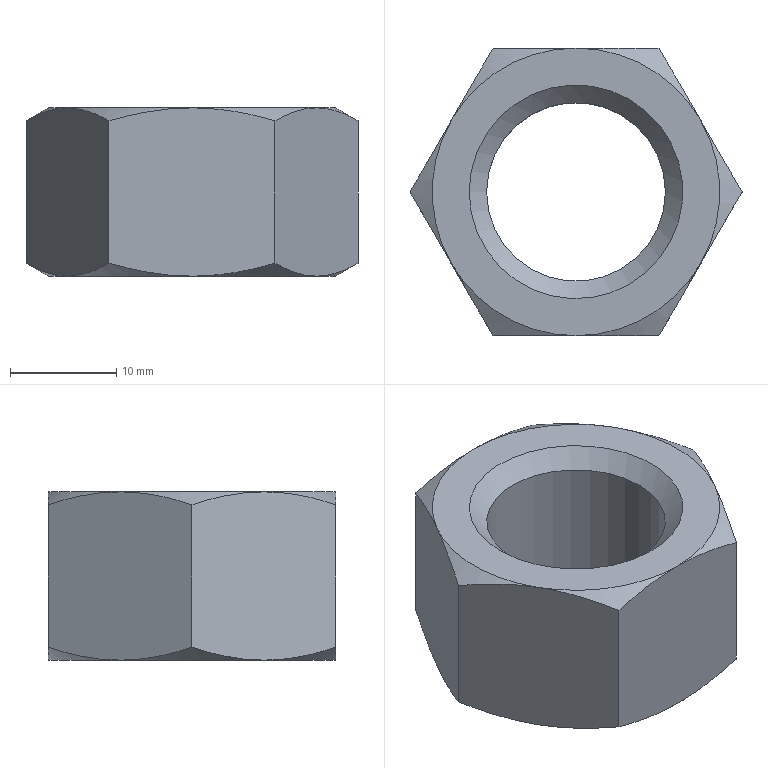Part | NX | features META 3, SKETCH 3, DATUM_CSYS 2, EXTRUDE 2, SWP104 2, CHAMFER 1, LINE 1, SYMBOLIC_THREAD 1, THREADS 1 | 1 solid | 23 faces | box 31.177 x 27 x 15.8 mm | volume 6286 mm3 | cone 14 | plane 8 | cylinder 1 | commonest cylinder face diameters 16.782 x1
STEP:
#1=CARTESIAN_POINT('',(-7.794,13.5,14.594));
#2=VERTEX_POINT('',#1);
#3=CARTESIAN_POINT('',(-7.794,13.5,1.206));
#4=VERTEX_POINT('',#3);
#5=CARTESIAN_POINT('',(-7.794,13.5,15.8));
#6=DIRECTION('',(0.,0.,-1.));
#7=VECTOR('',#6,1000.);
#8=LINE('',#5,#7);
#9=EDGE_CURVE('',#2,#4,#8,.T.);
#10=ORIENTED_EDGE('',*,*,#9,.T.);
#11=CARTESIAN_POINT('',(-11.691,6.75,0.));
#12=VERTEX_POINT('',#11);
#13=CARTESIAN_POINT('',(-7.794,13.5,1.206));
#14=CARTESIAN_POINT('',(-9.069,11.292,0.4696));
#15=CARTESIAN_POINT('',(-10.363,9.05,0.));
#16=CARTESIAN_POINT('',(-11.691,6.75,0.));
#17=B_SPLINE_CURVE_WITH_KNOTS('',3,(#13,#14,#15,#16),.UNSPECIFIED.,.F.,.F.,(4,4),(0.000000238,0.007887),.UNSPECIFIED.);
#18=EDGE_CURVE('',#4,#12,#17,.T.);
#19=ORIENTED_EDGE('',*,*,#18,.T.);
#20=CARTESIAN_POINT('',(-15.588,0.,1.206));
#21=VERTEX_POINT('',#20);
#22=CARTESIAN_POINT('',(-11.691,6.75,0.));
#23=CARTESIAN_POINT('',(-13.014,4.459,0.));
#24=CARTESIAN_POINT('',(-14.317,2.203,0.4715));
#25=CARTESIAN_POINT('',(-15.588,0.,1.206));
#26=B_SPLINE_CURVE_WITH_KNOTS('',3,(#22,#23,#24,#25),.UNSPECIFIED.,.F.,.F.,(4,4),(0.007887,0.01574),.UNSPECIFIED.);
#27=EDGE_CURVE('',#12,#21,#26,.T.);
#28=ORIENTED_EDGE('',*,*,#27,.T.);
#29=CARTESIAN_POINT('',(-15.588,0.,14.594));
#30=VERTEX_POINT('',#29);
#31=CARTESIAN_POINT('',(-15.588,0.,15.8));
#32=DIRECTION('',(0.,0.,-1.));
#33=VECTOR('',#32,1000.);
#34=LINE('',#31,#33);
#35=EDGE_CURVE('',#30,#21,#34,.T.);
#36=ORIENTED_EDGE('',*,*,#35,.F.);
#37=CARTESIAN_POINT('',(-11.691,6.75,15.8));
#38=VERTEX_POINT('',#37);
#39=CARTESIAN_POINT('',(-11.691,6.75,15.8));
#40=CARTESIAN_POINT('',(-13.014,4.459,15.8));
#41=CARTESIAN_POINT('',(-14.317,2.203,15.329));
#42=CARTESIAN_POINT('',(-15.588,0.,14.594));
#43=B_SPLINE_CURVE_WITH_KNOTS('',3,(#39,#40,#41,#42),.UNSPECIFIED.,.F.,.F.,(4,4),(0.007887,0.01574),.UNSPECIFIED.);
#44=EDGE_CURVE('',#38,#30,#43,.T.);
#45=ORIENTED_EDGE('',*,*,#44,.F.);
#46=CARTESIAN_POINT('',(-7.794,13.5,14.594));
#47=CARTESIAN_POINT('',(-9.069,11.292,15.33));
#48=CARTESIAN_POINT('',(-10.363,9.05,15.8));
#49=CARTESIAN_POINT('',(-11.691,6.75,15.8));
#50=B_SPLINE_CURVE_WITH_KNOTS('',3,(#46,#47,#48,#49),.UNSPECIFIED.,.F.,.F.,(4,4),(0.000000238,0.007887),.UNSPECIFIED.);
#51=EDGE_CURVE('',#2,#38,#50,.T.);
#52=ORIENTED_EDGE('',*,*,#51,.F.);
#53=EDGE_LOOP('',(#10,#19,#28,#36,#45,#52));
#54=FACE_BOUND('',#53,.T.);
#55=CARTESIAN_POINT('',(-15.588,0.,15.8));
#56=DIRECTION('',(-0.866,0.5,0.));
#57=DIRECTION('',(-0.5,-0.866,0.));
#58=AXIS2_PLACEMENT_3D('',#55,#56,#57);
#59=PLANE('',#58);
#60=ADVANCED_FACE('',(#54),#59,.T.);
#61=CARTESIAN_POINT('',(7.794,13.5,14.594));
#62=VERTEX_POINT('',#61);
#63=CARTESIAN_POINT('',(7.794,13.5,1.206));
#64=VERTEX_POINT('',#63);
#65=CARTESIAN_POINT('',(7.794,13.5,15.8));
#66=DIRECTION('',(0.,0.,-1.));
#67=VECTOR('',#66,1000.);
#68=LINE('',#65,#67);
#69=EDGE_CURVE('',#62,#64,#68,.T.);
#70=ORIENTED_EDGE('',*,*,#69,.T.);
#71=CARTESIAN_POINT('',(0.,13.5,0.));
#72=VERTEX_POINT('',#71);
#73=CARTESIAN_POINT('',(0.,13.5,0.));
#74=CARTESIAN_POINT('',(2.636,13.5,0.));
#75=CARTESIAN_POINT('',(5.274,13.5,0.4781));
#76=CARTESIAN_POINT('',(7.794,13.5,1.206));
#77=B_SPLINE_CURVE_WITH_KNOTS('',3,(#73,#74,#75,#76),.UNSPECIFIED.,.F.,.F.,(4,4),(0.02179,0.02968),.UNSPECIFIED.);
#78=EDGE_CURVE('',#64,#72,#77,.F.);
#79=ORIENTED_EDGE('',*,*,#78,.T.);
#80=CARTESIAN_POINT('',(-7.794,13.5,1.206));
#81=CARTESIAN_POINT('',(-5.259,13.5,0.4739));
#82=CARTESIAN_POINT('',(-2.634,13.5,0.));
#83=CARTESIAN_POINT('',(0.,13.5,0.));
#84=B_SPLINE_CURVE_WITH_KNOTS('',3,(#80,#81,#82,#83),.UNSPECIFIED.,.F.,.F.,(4,4),(0.01391,0.02179),.UNSPECIFIED.);
#85=EDGE_CURVE('',#72,#4,#84,.F.);
#86=ORIENTED_EDGE('',*,*,#85,.T.);
#87=ORIENTED_EDGE('',*,*,#9,.F.);
#88=CARTESIAN_POINT('',(0.,13.5,15.8));
#89=VERTEX_POINT('',#88);
#90=CARTESIAN_POINT('',(-7.794,13.5,14.594));
#91=CARTESIAN_POINT('',(-5.259,13.5,15.326));
#92=CARTESIAN_POINT('',(-2.634,13.5,15.8));
#93=CARTESIAN_POINT('',(0.,13.5,15.8));
#94=B_SPLINE_CURVE_WITH_KNOTS('',3,(#90,#91,#92,#93),.UNSPECIFIED.,.F.,.F.,(4,4),(0.01391,0.02179),.UNSPECIFIED.);
#95=EDGE_CURVE('',#89,#2,#94,.F.);
#96=ORIENTED_EDGE('',*,*,#95,.F.);
#97=CARTESIAN_POINT('',(0.,13.5,15.8));
#98=CARTESIAN_POINT('',(2.636,13.5,15.8));
#99=CARTESIAN_POINT('',(5.274,13.5,15.322));
#100=CARTESIAN_POINT('',(7.794,13.5,14.594));
#101=B_SPLINE_CURVE_WITH_KNOTS('',3,(#97,#98,#99,#100),.UNSPECIFIED.,.F.,.F.,(4,4),(0.02179,0.02968),.UNSPECIFIED.);
#102=EDGE_CURVE('',#62,#89,#101,.F.);
#103=ORIENTED_EDGE('',*,*,#102,.F.);
#104=EDGE_LOOP('',(#70,#79,#86,#87,#96,#103));
#105=FACE_BOUND('',#104,.T.);
#106=CARTESIAN_POINT('',(-7.794,13.5,15.8));
#107=DIRECTION('',(0.,1.,0.));
#108=DIRECTION('',(0.,0.,1.));
#109=AXIS2_PLACEMENT_3D('',#106,#107,#108);
#110=PLANE('',#109);
#111=ADVANCED_FACE('',(#105),#110,.T.);
#112=CARTESIAN_POINT('',(15.588,0.,14.594));
#113=VERTEX_POINT('',#112);
#114=CARTESIAN_POINT('',(15.588,0.,1.206));
#115=VERTEX_POINT('',#114);
#116=CARTESIAN_POINT('',(15.588,0.,15.8));
#117=DIRECTION('',(0.,0.,-1.));
#118=VECTOR('',#117,1000.);
#119=LINE('',#116,#118);
#120=EDGE_CURVE('',#113,#115,#119,.T.);
#121=ORIENTED_EDGE('',*,*,#120,.T.);
#122=CARTESIAN_POINT('',(11.691,6.75,0.));
#123=VERTEX_POINT('',#122);
#124=CARTESIAN_POINT('',(15.588,0.,1.206));
#125=CARTESIAN_POINT('',(14.313,2.208,0.4696));
#126=CARTESIAN_POINT('',(13.019,4.45,0.));
#127=CARTESIAN_POINT('',(11.691,6.75,0.));
#128=B_SPLINE_CURVE_WITH_KNOTS('',3,(#124,#125,#126,#127),.UNSPECIFIED.,.F.,.F.,(4,4),(0.000000238,0.007887),.UNSPECIFIED.);
#129=EDGE_CURVE('',#115,#123,#128,.T.);
#130=ORIENTED_EDGE('',*,*,#129,.T.);
#131=CARTESIAN_POINT('',(11.691,6.75,0.));
#132=CARTESIAN_POINT('',(10.368,9.041,0.));
#133=CARTESIAN_POINT('',(9.066,11.297,0.4715));
#134=CARTESIAN_POINT('',(7.794,13.5,1.206));
#135=B_SPLINE_CURVE_WITH_KNOTS('',3,(#131,#132,#133,#134),.UNSPECIFIED.,.F.,.F.,(4,4),(0.007887,0.01574),.UNSPECIFIED.);
#136=EDGE_CURVE('',#123,#64,#135,.T.);
#137=ORIENTED_EDGE('',*,*,#136,.T.);
#138=ORIENTED_EDGE('',*,*,#69,.F.);
#139=CARTESIAN_POINT('',(11.691,6.75,15.8));
#140=VERTEX_POINT('',#139);
#141=CARTESIAN_POINT('',(11.691,6.75,15.8));
#142=CARTESIAN_POINT('',(10.368,9.041,15.8));
#143=CARTESIAN_POINT('',(9.066,11.297,15.329));
#144=CARTESIAN_POINT('',(7.794,13.5,14.594));
#145=B_SPLINE_CURVE_WITH_KNOTS('',3,(#141,#142,#143,#144),.UNSPECIFIED.,.F.,.F.,(4,4),(0.007887,0.01574),.UNSPECIFIED.);
#146=EDGE_CURVE('',#140,#62,#145,.T.);
#147=ORIENTED_EDGE('',*,*,#146,.F.);
#148=CARTESIAN_POINT('',(15.588,0.,14.594));
#149=CARTESIAN_POINT('',(14.313,2.208,15.33));
#150=CARTESIAN_POINT('',(13.019,4.45,15.8));
#151=CARTESIAN_POINT('',(11.691,6.75,15.8));
#152=B_SPLINE_CURVE_WITH_KNOTS('',3,(#148,#149,#150,#151),.UNSPECIFIED.,.F.,.F.,(4,4),(0.000000238,0.007887),.UNSPECIFIED.);
#153=EDGE_CURVE('',#113,#140,#152,.T.);
#154=ORIENTED_EDGE('',*,*,#153,.F.);
#155=EDGE_LOOP('',(#121,#130,#137,#138,#147,#154));
#156=FACE_BOUND('',#155,.T.);
#157=CARTESIAN_POINT('',(7.794,13.5,15.8));
#158=DIRECTION('',(0.866,0.5,0.));
#159=DIRECTION('',(-0.5,0.866,0.));
#160=AXIS2_PLACEMENT_3D('',#157,#158,#159);
#161=PLANE('',#160);
#162=ADVANCED_FACE('',(#156),#161,.T.);
#163=CARTESIAN_POINT('',(7.794,-13.5,14.594));
#164=VERTEX_POINT('',#163);
#165=CARTESIAN_POINT('',(7.794,-13.5,1.206));
#166=VERTEX_POINT('',#165);
#167=CARTESIAN_POINT('',(7.794,-13.5,15.8));
#168=DIRECTION('',(0.,0.,-1.));
#169=VECTOR('',#168,1000.);
#170=LINE('',#167,#169);
#171=EDGE_CURVE('',#164,#166,#170,.T.);
#172=ORIENTED_EDGE('',*,*,#171,.T.);
#173=CARTESIAN_POINT('',(11.691,-6.75,0.));
#174=VERTEX_POINT('',#173);
#175=CARTESIAN_POINT('',(7.794,-13.5,1.206));
#176=CARTESIAN_POINT('',(9.069,-11.292,0.4696));
#177=CARTESIAN_POINT('',(10.363,-9.05,0.));
#178=CARTESIAN_POINT('',(11.691,-6.75,0.));
#179=B_SPLINE_CURVE_WITH_KNOTS('',3,(#175,#176,#177,#178),.UNSPECIFIED.,.F.,.F.,(4,4),(0.000000238,0.007887),.UNSPECIFIED.);
#180=EDGE_CURVE('',#166,#174,#179,.T.);
#181=ORIENTED_EDGE('',*,*,#180,.T.);
#182=CARTESIAN_POINT('',(11.691,-6.75,0.));
#183=CARTESIAN_POINT('',(13.014,-4.459,0.));
#184=CARTESIAN_POINT('',(14.317,-2.203,0.4715));
#185=CARTESIAN_POINT('',(15.588,0.,1.206));
#186=B_SPLINE_CURVE_WITH_KNOTS('',3,(#182,#183,#184,#185),.UNSPECIFIED.,.F.,.F.,(4,4),(0.007887,0.01574),.UNSPECIFIED.);
#187=EDGE_CURVE('',#174,#115,#186,.T.);
#188=ORIENTED_EDGE('',*,*,#187,.T.);
#189=ORIENTED_EDGE('',*,*,#120,.F.);
#190=CARTESIAN_POINT('',(11.691,-6.75,15.8));
#191=VERTEX_POINT('',#190);
#192=CARTESIAN_POINT('',(11.691,-6.75,15.8));
#193=CARTESIAN_POINT('',(13.014,-4.459,15.8));
#194=CARTESIAN_POINT('',(14.317,-2.203,15.329));
#195=CARTESIAN_POINT('',(15.588,0.,14.594));
#196=B_SPLINE_CURVE_WITH_KNOTS('',3,(#192,#193,#194,#195),.UNSPECIFIED.,.F.,.F.,(4,4),(0.007887,0.01574),.UNSPECIFIED.);
#197=EDGE_CURVE('',#191,#113,#196,.T.);
#198=ORIENTED_EDGE('',*,*,#197,.F.);
#199=CARTESIAN_POINT('',(7.794,-13.5,14.594));
#200=CARTESIAN_POINT('',(9.069,-11.292,15.33));
#201=CARTESIAN_POINT('',(10.363,-9.05,15.8));
#202=CARTESIAN_POINT('',(11.691,-6.75,15.8));
#203=B_SPLINE_CURVE_WITH_KNOTS('',3,(#199,#200,#201,#202),.UNSPECIFIED.,.F.,.F.,(4,4),(0.000000238,0.007887),.UNSPECIFIED.);
#204=EDGE_CURVE('',#164,#191,#203,.T.);
#205=ORIENTED_EDGE('',*,*,#204,.F.);
#206=EDGE_LOOP('',(#172,#181,#188,#189,#198,#205));
#207=FACE_BOUND('',#206,.T.);
#208=CARTESIAN_POINT('',(15.588,0.,15.8));
#209=DIRECTION('',(0.866,-0.5,0.));
#210=DIRECTION('',(0.5,0.866,0.));
#211=AXIS2_PLACEMENT_3D('',#208,#209,#210);
#212=PLANE('',#211);
#213=ADVANCED_FACE('',(#207),#212,.T.);
#214=CARTESIAN_POINT('',(-7.794,-13.5,14.594));
#215=VERTEX_POINT('',#214);
#216=CARTESIAN_POINT('',(-7.794,-13.5,1.206));
#217=VERTEX_POINT('',#216);
#218=CARTESIAN_POINT('',(-7.794,-13.5,15.8));
#219=DIRECTION('',(0.,0.,-1.));
#220=VECTOR('',#219,1000.);
#221=LINE('',#218,#220);
#222=EDGE_CURVE('',#215,#217,#221,.T.);
#223=ORIENTED_EDGE('',*,*,#222,.T.);
#224=CARTESIAN_POINT('',(0.,-13.5,0.));
#225=VERTEX_POINT('',#224);
#226=CARTESIAN_POINT('',(-7.794,-13.5,1.206));
#227=CARTESIAN_POINT('',(-5.259,-13.5,0.4739));
#228=CARTESIAN_POINT('',(-2.634,-13.5,0.));
#229=CARTESIAN_POINT('',(0.,-13.5,0.));
#230=B_SPLINE_CURVE_WITH_KNOTS('',3,(#226,#227,#228,#229),.UNSPECIFIED.,.F.,.F.,(4,4),(0.01391,0.02179),.UNSPECIFIED.);
#231=EDGE_CURVE('',#217,#225,#230,.T.);
#232=ORIENTED_EDGE('',*,*,#231,.T.);
#233=CARTESIAN_POINT('',(0.,-13.5,0.));
#234=CARTESIAN_POINT('',(2.636,-13.5,0.));
#235=CARTESIAN_POINT('',(5.274,-13.5,0.4781));
#236=CARTESIAN_POINT('',(7.794,-13.5,1.206));
#237=B_SPLINE_CURVE_WITH_KNOTS('',3,(#233,#234,#235,#236),.UNSPECIFIED.,.F.,.F.,(4,4),(0.02179,0.02968),.UNSPECIFIED.);
#238=EDGE_CURVE('',#225,#166,#237,.T.);
#239=ORIENTED_EDGE('',*,*,#238,.T.);
#240=ORIENTED_EDGE('',*,*,#171,.F.);
#241=CARTESIAN_POINT('',(0.,-13.5,15.8));
#242=VERTEX_POINT('',#241);
#243=CARTESIAN_POINT('',(0.,-13.5,15.8));
#244=CARTESIAN_POINT('',(2.636,-13.5,15.8));
#245=CARTESIAN_POINT('',(5.274,-13.5,15.322));
#246=CARTESIAN_POINT('',(7.794,-13.5,14.594));
#247=B_SPLINE_CURVE_WITH_KNOTS('',3,(#243,#244,#245,#246),.UNSPECIFIED.,.F.,.F.,(4,4),(0.02179,0.02968),.UNSPECIFIED.);
#248=EDGE_CURVE('',#242,#164,#247,.T.);
#249=ORIENTED_EDGE('',*,*,#248,.F.);
#250=CARTESIAN_POINT('',(-7.794,-13.5,14.594));
#251=CARTESIAN_POINT('',(-5.259,-13.5,15.326));
#252=CARTESIAN_POINT('',(-2.634,-13.5,15.8));
#253=CARTESIAN_POINT('',(0.,-13.5,15.8));
#254=B_SPLINE_CURVE_WITH_KNOTS('',3,(#250,#251,#252,#253),.UNSPECIFIED.,.F.,.F.,(4,4),(0.01391,0.02179),.UNSPECIFIED.);
#255=EDGE_CURVE('',#215,#242,#254,.T.);
#256=ORIENTED_EDGE('',*,*,#255,.F.);
#257=EDGE_LOOP('',(#223,#232,#239,#240,#249,#256));
#258=FACE_BOUND('',#257,.T.);
#259=CARTESIAN_POINT('',(7.794,-13.5,15.8));
#260=DIRECTION('',(0.,-1.,0.));
#261=DIRECTION('',(0.,0.,-1.));
#262=AXIS2_PLACEMENT_3D('',#259,#260,#261);
#263=PLANE('',#262);
#264=ADVANCED_FACE('',(#258),#263,.T.);
#265=ORIENTED_EDGE('',*,*,#35,.T.);
#266=CARTESIAN_POINT('',(-11.691,-6.75,0.));
#267=VERTEX_POINT('',#266);
#268=CARTESIAN_POINT('',(-15.588,0.,1.206));
#269=CARTESIAN_POINT('',(-14.313,-2.208,0.4696));
#270=CARTESIAN_POINT('',(-13.019,-4.45,0.));
#271=CARTESIAN_POINT('',(-11.691,-6.75,0.));
#272=B_SPLINE_CURVE_WITH_KNOTS('',3,(#268,#269,#270,#271),.UNSPECIFIED.,.F.,.F.,(4,4),(0.000000238,0.007887),.UNSPECIFIED.);
#273=EDGE_CURVE('',#21,#267,#272,.T.);
#274=ORIENTED_EDGE('',*,*,#273,.T.);
#275=CARTESIAN_POINT('',(-11.691,-6.75,0.));
#276=CARTESIAN_POINT('',(-10.368,-9.041,0.));
#277=CARTESIAN_POINT('',(-9.066,-11.297,0.4715));
#278=CARTESIAN_POINT('',(-7.794,-13.5,1.206));
#279=B_SPLINE_CURVE_WITH_KNOTS('',3,(#275,#276,#277,#278),.UNSPECIFIED.,.F.,.F.,(4,4),(0.007887,0.01574),.UNSPECIFIED.);
#280=EDGE_CURVE('',#267,#217,#279,.T.);
#281=ORIENTED_EDGE('',*,*,#280,.T.);
#282=ORIENTED_EDGE('',*,*,#222,.F.);
#283=CARTESIAN_POINT('',(-11.691,-6.75,15.8));
#284=VERTEX_POINT('',#283);
#285=CARTESIAN_POINT('',(-11.691,-6.75,15.8));
#286=CARTESIAN_POINT('',(-10.368,-9.041,15.8));
#287=CARTESIAN_POINT('',(-9.066,-11.297,15.329));
#288=CARTESIAN_POINT('',(-7.794,-13.5,14.594));
#289=B_SPLINE_CURVE_WITH_KNOTS('',3,(#285,#286,#287,#288),.UNSPECIFIED.,.F.,.F.,(4,4),(0.007887,0.01574),.UNSPECIFIED.);
#290=EDGE_CURVE('',#284,#215,#289,.T.);
#291=ORIENTED_EDGE('',*,*,#290,.F.);
#292=CARTESIAN_POINT('',(-15.588,0.,14.594));
#293=CARTESIAN_POINT('',(-14.313,-2.208,15.33));
#294=CARTESIAN_POINT('',(-13.019,-4.45,15.8));
#295=CARTESIAN_POINT('',(-11.691,-6.75,15.8));
#296=B_SPLINE_CURVE_WITH_KNOTS('',3,(#292,#293,#294,#295),.UNSPECIFIED.,.F.,.F.,(4,4),(0.000000238,0.007887),.UNSPECIFIED.);
#297=EDGE_CURVE('',#30,#284,#296,.T.);
#298=ORIENTED_EDGE('',*,*,#297,.F.);
#299=EDGE_LOOP('',(#265,#274,#281,#282,#291,#298));
#300=FACE_BOUND('',#299,.T.);
#301=CARTESIAN_POINT('',(-7.794,-13.5,15.8));
#302=DIRECTION('',(-0.866,-0.5,0.));
#303=DIRECTION('',(0.5,-0.866,0.));
#304=AXIS2_PLACEMENT_3D('',#301,#302,#303);
#305=PLANE('',#304);
#306=ADVANCED_FACE('',(#300),#305,.T.);
#307=CARTESIAN_POINT('',(-10.027,0.,0.));
#308=VERTEX_POINT('',#307);
#309=CARTESIAN_POINT('',(0.,0.,0.));
#310=DIRECTION('',(0.,0.,-1.));
#311=DIRECTION('',(-1.,0.,0.));
#312=AXIS2_PLACEMENT_3D('',#309,#310,#311);
#313=CIRCLE('',#312,10.027);
#314=EDGE_CURVE('',#308,#308,#313,.F.);
#315=ORIENTED_EDGE('',*,*,#314,.T.);
#316=EDGE_LOOP('',(#315));
#317=FACE_BOUND('',#316,.T.);
#318=CARTESIAN_POINT('',(0.,0.,0.));
#319=DIRECTION('',(0.,0.,-1.));
#320=DIRECTION('',(-1.,0.,0.));
#321=AXIS2_PLACEMENT_3D('',#318,#319,#320);
#322=CIRCLE('',#321,13.5);
#323=EDGE_CURVE('',#267,#12,#322,.T.);
#324=ORIENTED_EDGE('',*,*,#323,.T.);
#325=CARTESIAN_POINT('',(0.,0.,0.));
#326=DIRECTION('',(0.,0.,-1.));
#327=DIRECTION('',(-1.,0.,0.));
#328=AXIS2_PLACEMENT_3D('',#325,#326,#327);
#329=CIRCLE('',#328,13.5);
#330=EDGE_CURVE('',#12,#72,#329,.T.);
#331=ORIENTED_EDGE('',*,*,#330,.T.);
#332=CARTESIAN_POINT('',(0.,0.,0.));
#333=DIRECTION('',(0.,0.,-1.));
#334=DIRECTION('',(-1.,0.,0.));
#335=AXIS2_PLACEMENT_3D('',#332,#333,#334);
#336=CIRCLE('',#335,13.5);
#337=EDGE_CURVE('',#72,#123,#336,.T.);
#338=ORIENTED_EDGE('',*,*,#337,.T.);
#339=CARTESIAN_POINT('',(0.,0.,0.));
#340=DIRECTION('',(0.,0.,-1.));
#341=DIRECTION('',(-1.,0.,0.));
#342=AXIS2_PLACEMENT_3D('',#339,#340,#341);
#343=CIRCLE('',#342,13.5);
#344=EDGE_CURVE('',#123,#174,#343,.T.);
#345=ORIENTED_EDGE('',*,*,#344,.T.);
#346=CARTESIAN_POINT('',(0.,0.,0.));
#347=DIRECTION('',(0.,0.,-1.));
#348=DIRECTION('',(-1.,0.,0.));
#349=AXIS2_PLACEMENT_3D('',#346,#347,#348);
#350=CIRCLE('',#349,13.5);
#351=EDGE_CURVE('',#174,#225,#350,.T.);
#352=ORIENTED_EDGE('',*,*,#351,.T.);
#353=CARTESIAN_POINT('',(0.,0.,0.));
#354=DIRECTION('',(0.,0.,-1.));
#355=DIRECTION('',(-1.,0.,0.));
#356=AXIS2_PLACEMENT_3D('',#353,#354,#355);
#357=CIRCLE('',#356,13.5);
#358=EDGE_CURVE('',#225,#267,#357,.T.);
#359=ORIENTED_EDGE('',*,*,#358,.T.);
#360=EDGE_LOOP('',(#324,#331,#338,#345,#352,#359));
#361=FACE_BOUND('',#360,.T.);
#362=CARTESIAN_POINT('',(-7.794,13.5,0.));
#363=DIRECTION('',(0.,0.,-1.));
#364=DIRECTION('',(-1.,0.,0.));
#365=AXIS2_PLACEMENT_3D('',#362,#363,#364);
#366=PLANE('',#365);
#367=ADVANCED_FACE('',(#317,#361),#366,.T.);
#368=CARTESIAN_POINT('',(-10.027,0.,15.8));
#369=VERTEX_POINT('',#368);
#370=CARTESIAN_POINT('',(0.,0.,15.8));
#371=DIRECTION('',(0.,0.,-1.));
#372=DIRECTION('',(-1.,0.,0.));
#373=AXIS2_PLACEMENT_3D('',#370,#371,#372);
#374=CIRCLE('',#373,10.027);
#375=EDGE_CURVE('',#369,#369,#374,.T.);
#376=ORIENTED_EDGE('',*,*,#375,.T.);
#377=EDGE_LOOP('',(#376));
#378=FACE_BOUND('',#377,.T.);
#379=CARTESIAN_POINT('',(0.,0.,15.8));
#380=DIRECTION('',(0.,0.,-1.));
#381=DIRECTION('',(-1.,0.,0.));
#382=AXIS2_PLACEMENT_3D('',#379,#380,#381);
#383=CIRCLE('',#382,13.5);
#384=EDGE_CURVE('',#38,#89,#383,.T.);
#385=ORIENTED_EDGE('',*,*,#384,.F.);
#386=CARTESIAN_POINT('',(0.,0.,15.8));
#387=DIRECTION('',(0.,0.,-1.));
#388=DIRECTION('',(-1.,0.,0.));
#389=AXIS2_PLACEMENT_3D('',#386,#387,#388);
#390=CIRCLE('',#389,13.5);
#391=EDGE_CURVE('',#284,#38,#390,.T.);
#392=ORIENTED_EDGE('',*,*,#391,.F.);
#393=CARTESIAN_POINT('',(0.,0.,15.8));
#394=DIRECTION('',(0.,0.,-1.));
#395=DIRECTION('',(-1.,0.,0.));
#396=AXIS2_PLACEMENT_3D('',#393,#394,#395);
#397=CIRCLE('',#396,13.5);
#398=EDGE_CURVE('',#242,#284,#397,.T.);
#399=ORIENTED_EDGE('',*,*,#398,.F.);
#400=CARTESIAN_POINT('',(0.,0.,15.8));
#401=DIRECTION('',(0.,0.,-1.));
#402=DIRECTION('',(-1.,0.,0.));
#403=AXIS2_PLACEMENT_3D('',#400,#401,#402);
#404=CIRCLE('',#403,13.5);
#405=EDGE_CURVE('',#191,#242,#404,.T.);
#406=ORIENTED_EDGE('',*,*,#405,.F.);
#407=CARTESIAN_POINT('',(0.,0.,15.8));
#408=DIRECTION('',(0.,0.,-1.));
#409=DIRECTION('',(-1.,0.,0.));
#410=AXIS2_PLACEMENT_3D('',#407,#408,#409);
#411=CIRCLE('',#410,13.5);
#412=EDGE_CURVE('',#140,#191,#411,.T.);
#413=ORIENTED_EDGE('',*,*,#412,.F.);
#414=CARTESIAN_POINT('',(0.,0.,15.8));
#415=DIRECTION('',(0.,0.,-1.));
#416=DIRECTION('',(-1.,0.,0.));
#417=AXIS2_PLACEMENT_3D('',#414,#415,#416);
#418=CIRCLE('',#417,13.5);
#419=EDGE_CURVE('',#89,#140,#418,.T.);
#420=ORIENTED_EDGE('',*,*,#419,.F.);
#421=EDGE_LOOP('',(#385,#392,#399,#406,#413,#420));
#422=FACE_BOUND('',#421,.T.);
#423=CARTESIAN_POINT('',(-7.794,13.5,15.8));
#424=DIRECTION('',(0.,0.,-1.));
#425=DIRECTION('',(-1.,0.,0.));
#426=AXIS2_PLACEMENT_3D('',#423,#424,#425);
#427=PLANE('',#426);
#428=ADVANCED_FACE('',(#378,#422),#427,.F.);
#429=CARTESIAN_POINT('',(-8.391,0.,1.635));
#430=VERTEX_POINT('',#429);
#431=CARTESIAN_POINT('',(0.,0.,1.635));
#432=DIRECTION('',(0.,0.,-1.));
#433=DIRECTION('',(-1.,0.,0.));
#434=AXIS2_PLACEMENT_3D('',#431,#432,#433);
#435=CIRCLE('',#434,8.391);
#436=EDGE_CURVE('',#430,#430,#435,.T.);
#437=ORIENTED_EDGE('',*,*,#436,.T.);
#438=EDGE_LOOP('',(#437));
#439=FACE_BOUND('',#438,.T.);
#440=CARTESIAN_POINT('',(-8.391,0.,14.165));
#441=VERTEX_POINT('',#440);
#442=CARTESIAN_POINT('',(0.,0.,14.165));
#443=DIRECTION('',(0.,0.,-1.));
#444=DIRECTION('',(-1.,0.,0.));
#445=AXIS2_PLACEMENT_3D('',#442,#443,#444);
#446=CIRCLE('',#445,8.391);
#447=EDGE_CURVE('',#441,#441,#446,.F.);
#448=ORIENTED_EDGE('',*,*,#447,.T.);
#449=EDGE_LOOP('',(#448));
#450=FACE_BOUND('',#449,.T.);
#451=CARTESIAN_POINT('',(0.,0.,15.8));
#452=DIRECTION('',(0.,0.,-1.));
#453=DIRECTION('',(-1.,0.,0.));
#454=AXIS2_PLACEMENT_3D('',#451,#452,#453);
#455=CYLINDRICAL_SURFACE('',#454,8.391);
#456=ADVANCED_FACE('',(#439,#450),#455,.F.);
#457=ORIENTED_EDGE('',*,*,#255,.T.);
#458=ORIENTED_EDGE('',*,*,#398,.T.);
#459=ORIENTED_EDGE('',*,*,#290,.T.);
#460=EDGE_LOOP('',(#457,#458,#459));
#461=FACE_BOUND('',#460,.T.);
#462=CARTESIAN_POINT('',(0.,0.,15.8));
#463=DIRECTION('',(0.,0.,-1.));
#464=DIRECTION('',(-1.,0.,0.));
#465=AXIS2_PLACEMENT_3D('',#462,#463,#464);
#466=CONICAL_SURFACE('',#465,13.5,1.047);
#467=ADVANCED_FACE('',(#461),#466,.T.);
#468=ORIENTED_EDGE('',*,*,#44,.T.);
#469=ORIENTED_EDGE('',*,*,#297,.T.);
#470=ORIENTED_EDGE('',*,*,#391,.T.);
#471=EDGE_LOOP('',(#468,#469,#470));
#472=FACE_BOUND('',#471,.T.);
#473=CARTESIAN_POINT('',(0.,0.,15.8));
#474=DIRECTION('',(0.,0.,-1.));
#475=DIRECTION('',(-1.,0.,0.));
#476=AXIS2_PLACEMENT_3D('',#473,#474,#475);
#477=CONICAL_SURFACE('',#476,13.5,1.047);
#478=ADVANCED_FACE('',(#472),#477,.T.);
#479=ORIENTED_EDGE('',*,*,#204,.T.);
#480=ORIENTED_EDGE('',*,*,#405,.T.);
#481=ORIENTED_EDGE('',*,*,#248,.T.);
#482=EDGE_LOOP('',(#479,#480,#481));
#483=FACE_BOUND('',#482,.T.);
#484=CARTESIAN_POINT('',(0.,0.,15.8));
#485=DIRECTION('',(0.,0.,-1.));
#486=DIRECTION('',(-1.,0.,0.));
#487=AXIS2_PLACEMENT_3D('',#484,#485,#486);
#488=CONICAL_SURFACE('',#487,13.5,1.047);
#489=ADVANCED_FACE('',(#483),#488,.T.);
#490=ORIENTED_EDGE('',*,*,#153,.T.);
#491=ORIENTED_EDGE('',*,*,#412,.T.);
#492=ORIENTED_EDGE('',*,*,#197,.T.);
#493=EDGE_LOOP('',(#490,#491,#492));
#494=FACE_BOUND('',#493,.T.);
#495=CARTESIAN_POINT('',(0.,0.,15.8));
#496=DIRECTION('',(0.,0.,-1.));
#497=DIRECTION('',(-1.,0.,0.));
#498=AXIS2_PLACEMENT_3D('',#495,#496,#497);
#499=CONICAL_SURFACE('',#498,13.5,1.047);
#500=ADVANCED_FACE('',(#494),#499,.T.);
#501=ORIENTED_EDGE('',*,*,#146,.T.);
#502=ORIENTED_EDGE('',*,*,#102,.T.);
#503=ORIENTED_EDGE('',*,*,#419,.T.);
#504=EDGE_LOOP('',(#501,#502,#503));
#505=FACE_BOUND('',#504,.T.);
#506=CARTESIAN_POINT('',(0.,0.,15.8));
#507=DIRECTION('',(0.,0.,-1.));
#508=DIRECTION('',(-1.,0.,0.));
#509=AXIS2_PLACEMENT_3D('',#506,#507,#508);
#510=CONICAL_SURFACE('',#509,13.5,1.047);
#511=ADVANCED_FACE('',(#505),#510,.T.);
#512=ORIENTED_EDGE('',*,*,#95,.T.);
#513=ORIENTED_EDGE('',*,*,#51,.T.);
#514=ORIENTED_EDGE('',*,*,#384,.T.);
#515=EDGE_LOOP('',(#512,#513,#514));
#516=FACE_BOUND('',#515,.T.);
#517=CARTESIAN_POINT('',(0.,0.,15.8));
#518=DIRECTION('',(0.,0.,-1.));
#519=DIRECTION('',(-1.,0.,0.));
#520=AXIS2_PLACEMENT_3D('',#517,#518,#519);
#521=CONICAL_SURFACE('',#520,13.5,1.047);
#522=ADVANCED_FACE('',(#516),#521,.T.);
#523=ORIENTED_EDGE('',*,*,#280,.F.);
#524=ORIENTED_EDGE('',*,*,#358,.F.);
#525=ORIENTED_EDGE('',*,*,#231,.F.);
#526=EDGE_LOOP('',(#523,#524,#525));
#527=FACE_BOUND('',#526,.T.);
#528=CARTESIAN_POINT('',(0.,0.,0.));
#529=DIRECTION('',(0.,0.,1.));
#530=DIRECTION('',(1.,0.,0.));
#531=AXIS2_PLACEMENT_3D('',#528,#529,#530);
#532=CONICAL_SURFACE('',#531,13.5,1.047);
#533=ADVANCED_FACE('',(#527),#532,.T.);
#534=ORIENTED_EDGE('',*,*,#323,.F.);
#535=ORIENTED_EDGE('',*,*,#273,.F.);
#536=ORIENTED_EDGE('',*,*,#27,.F.);
#537=EDGE_LOOP('',(#534,#535,#536));
#538=FACE_BOUND('',#537,.T.);
#539=CARTESIAN_POINT('',(0.,0.,0.));
#540=DIRECTION('',(0.,0.,1.));
#541=DIRECTION('',(1.,0.,0.));
#542=AXIS2_PLACEMENT_3D('',#539,#540,#541);
#543=CONICAL_SURFACE('',#542,13.5,1.047);
#544=ADVANCED_FACE('',(#538),#543,.T.);
#545=ORIENTED_EDGE('',*,*,#238,.F.);
#546=ORIENTED_EDGE('',*,*,#351,.F.);
#547=ORIENTED_EDGE('',*,*,#180,.F.);
#548=EDGE_LOOP('',(#545,#546,#547));
#549=FACE_BOUND('',#548,.T.);
#550=CARTESIAN_POINT('',(0.,0.,0.));
#551=DIRECTION('',(0.,0.,1.));
#552=DIRECTION('',(1.,0.,0.));
#553=AXIS2_PLACEMENT_3D('',#550,#551,#552);
#554=CONICAL_SURFACE('',#553,13.5,1.047);
#555=ADVANCED_FACE('',(#549),#554,.T.);
#556=ORIENTED_EDGE('',*,*,#187,.F.);
#557=ORIENTED_EDGE('',*,*,#344,.F.);
#558=ORIENTED_EDGE('',*,*,#129,.F.);
#559=EDGE_LOOP('',(#556,#557,#558));
#560=FACE_BOUND('',#559,.T.);
#561=CARTESIAN_POINT('',(0.,0.,0.));
#562=DIRECTION('',(0.,0.,1.));
#563=DIRECTION('',(1.,0.,0.));
#564=AXIS2_PLACEMENT_3D('',#561,#562,#563);
#565=CONICAL_SURFACE('',#564,13.5,1.047);
#566=ADVANCED_FACE('',(#560),#565,.T.);
#567=ORIENTED_EDGE('',*,*,#337,.F.);
#568=ORIENTED_EDGE('',*,*,#78,.F.);
#569=ORIENTED_EDGE('',*,*,#136,.F.);
#570=EDGE_LOOP('',(#567,#568,#569));
#571=FACE_BOUND('',#570,.T.);
#572=CARTESIAN_POINT('',(0.,0.,0.));
#573=DIRECTION('',(0.,0.,1.));
#574=DIRECTION('',(1.,0.,0.));
#575=AXIS2_PLACEMENT_3D('',#572,#573,#574);
#576=CONICAL_SURFACE('',#575,13.5,1.047);
#577=ADVANCED_FACE('',(#571),#576,.T.);
#578=ORIENTED_EDGE('',*,*,#330,.F.);
#579=ORIENTED_EDGE('',*,*,#18,.F.);
#580=ORIENTED_EDGE('',*,*,#85,.F.);
#581=EDGE_LOOP('',(#578,#579,#580));
#582=FACE_BOUND('',#581,.T.);
#583=CARTESIAN_POINT('',(0.,0.,0.));
#584=DIRECTION('',(0.,0.,1.));
#585=DIRECTION('',(1.,0.,0.));
#586=AXIS2_PLACEMENT_3D('',#583,#584,#585);
#587=CONICAL_SURFACE('',#586,13.5,1.047);
#588=ADVANCED_FACE('',(#582),#587,.T.);
#589=ORIENTED_EDGE('',*,*,#314,.F.);
#590=EDGE_LOOP('',(#589));
#591=FACE_BOUND('',#590,.T.);
#592=ORIENTED_EDGE('',*,*,#436,.F.);
#593=EDGE_LOOP('',(#592));
#594=FACE_BOUND('',#593,.T.);
#595=CARTESIAN_POINT('',(0.,0.,1.635));
#596=DIRECTION('',(0.,0.,-1.));
#597=DIRECTION('',(-1.,0.,0.));
#598=AXIS2_PLACEMENT_3D('',#595,#596,#597);
#599=CONICAL_SURFACE('',#598,8.391,0.7854);
#600=ADVANCED_FACE('',(#591,#594),#599,.F.);
#601=ORIENTED_EDGE('',*,*,#447,.F.);
#602=EDGE_LOOP('',(#601));
#603=FACE_BOUND('',#602,.T.);
#604=ORIENTED_EDGE('',*,*,#375,.F.);
#605=EDGE_LOOP('',(#604));
#606=FACE_BOUND('',#605,.T.);
#607=CARTESIAN_POINT('',(0.,0.,15.8));
#608=DIRECTION('',(0.,0.,1.));
#609=DIRECTION('',(1.,0.,0.));
#610=AXIS2_PLACEMENT_3D('',#607,#608,#609);
#611=CONICAL_SURFACE('',#610,10.027,0.7854);
#612=ADVANCED_FACE('',(#603,#606),#611,.F.);
#613=CLOSED_SHELL('',(#60,#111,#162,#213,#264,#306,#367,#428,#456,#467,#478,#489,#500,#511,#522,#533,#544,#555,#566,#577,#588,#600,#612));
#614=MANIFOLD_SOLID_BREP('',#613);
#615=(LENGTH_UNIT()NAMED_UNIT(*)SI_UNIT(.MILLI.,.METRE.));
#616=UNCERTAINTY_MEASURE_WITH_UNIT(LENGTH_MEASURE(0.0508),#615,'','');
#617=(NAMED_UNIT(*)PLANE_ANGLE_UNIT()SI_UNIT($,.RADIAN.));
#618=(NAMED_UNIT(*)SI_UNIT($,.STERADIAN.)SOLID_ANGLE_UNIT());
#619=(GEOMETRIC_REPRESENTATION_CONTEXT(3)GLOBAL_UNCERTAINTY_ASSIGNED_CONTEXT((#616))GLOBAL_UNIT_ASSIGNED_CONTEXT((#615,#617,#618))REPRESENTATION_CONTEXT('',''));
#620=ADVANCED_BREP_SHAPE_REPRESENTATION('',(#614),#619);